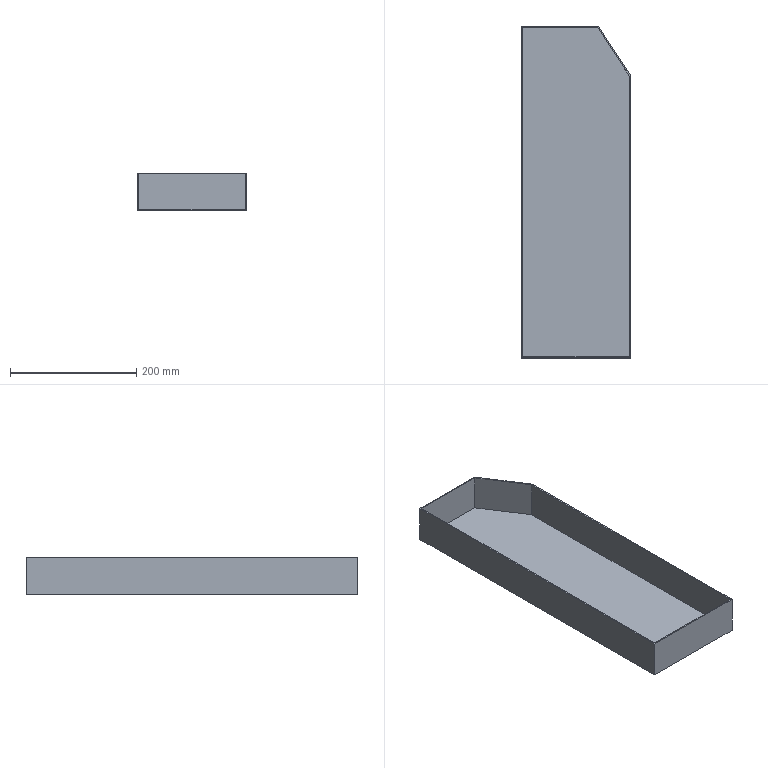Part | NX | features solid 2 | 1 solid | 13 faces | box 173 x 525 x 60 mm | volume 334513 mm3 | plane 13
STEP:
#1=CARTESIAN_POINT('',(730.,-500.,-255.));
#2=VERTEX_POINT('',#1);
#3=CARTESIAN_POINT('',(557.,-500.,-255.));
#4=VERTEX_POINT('',#3);
#5=CARTESIAN_POINT('',(-1080.,-500.,-255.));
#6=DIRECTION('',(1.,0.,0.));
#7=VECTOR('',#6,1000.);
#8=LINE('',#5,#7);
#9=EDGE_CURVE('',#2,#4,#8,.F.);
#10=ORIENTED_EDGE('',*,*,#9,.T.);
#11=CARTESIAN_POINT('',(557.,-500.,-315.));
#12=VERTEX_POINT('',#11);
#13=CARTESIAN_POINT('',(557.,-500.,-100.));
#14=DIRECTION('',(0.,0.,1.));
#15=VECTOR('',#14,1000.);
#16=LINE('',#13,#15);
#17=EDGE_CURVE('',#12,#4,#16,.T.);
#18=ORIENTED_EDGE('',*,*,#17,.F.);
#19=CARTESIAN_POINT('',(730.,-500.,-315.));
#20=VERTEX_POINT('',#19);
#21=CARTESIAN_POINT('',(-1080.,-500.,-315.));
#22=DIRECTION('',(1.,0.,0.));
#23=VECTOR('',#22,1000.);
#24=LINE('',#21,#23);
#25=EDGE_CURVE('',#20,#12,#24,.F.);
#26=ORIENTED_EDGE('',*,*,#25,.F.);
#27=CARTESIAN_POINT('',(730.,-500.,-315.));
#28=DIRECTION('',(0.,0.,1.));
#29=VECTOR('',#28,1000.);
#30=LINE('',#27,#29);
#31=EDGE_CURVE('',#20,#2,#30,.T.);
#32=ORIENTED_EDGE('',*,*,#31,.T.);
#33=EDGE_LOOP('',(#10,#18,#26,#32));
#34=FACE_BOUND('',#33,.T.);
#35=CARTESIAN_POINT('',(-1080.,-500.,-100.));
#36=DIRECTION('',(0.,1.,0.));
#37=DIRECTION('',(0.,0.,1.));
#38=AXIS2_PLACEMENT_3D('',#35,#36,#37);
#39=PLANE('',#38);
#40=ADVANCED_FACE('',(#34),#39,.F.);
#41=CARTESIAN_POINT('',(557.,25.,-255.));
#42=VERTEX_POINT('',#41);
#43=CARTESIAN_POINT('',(557.,-440.,-255.));
#44=DIRECTION('',(0.,1.,0.));
#45=VECTOR('',#44,1000.);
#46=LINE('',#43,#45);
#47=EDGE_CURVE('',#42,#4,#46,.F.);
#48=ORIENTED_EDGE('',*,*,#47,.F.);
#49=CARTESIAN_POINT('',(557.,25.,-315.));
#50=VERTEX_POINT('',#49);
#51=CARTESIAN_POINT('',(557.,25.,-315.));
#52=DIRECTION('',(0.,0.,1.));
#53=VECTOR('',#52,1000.);
#54=LINE('',#51,#53);
#55=EDGE_CURVE('',#50,#42,#54,.T.);
#56=ORIENTED_EDGE('',*,*,#55,.F.);
#57=CARTESIAN_POINT('',(557.,-440.,-315.));
#58=DIRECTION('',(0.,1.,0.));
#59=VECTOR('',#58,1000.);
#60=LINE('',#57,#59);
#61=EDGE_CURVE('',#50,#12,#60,.F.);
#62=ORIENTED_EDGE('',*,*,#61,.T.);
#63=ORIENTED_EDGE('',*,*,#17,.T.);
#64=EDGE_LOOP('',(#48,#56,#62,#63));
#65=FACE_BOUND('',#64,.T.);
#66=CARTESIAN_POINT('',(557.,-440.,-315.));
#67=DIRECTION('',(-1.,0.,0.));
#68=DIRECTION('',(0.,0.,1.));
#69=AXIS2_PLACEMENT_3D('',#66,#67,#68);
#70=PLANE('',#69);
#71=ADVANCED_FACE('',(#65),#70,.T.);
#72=CARTESIAN_POINT('',(678.942,25.,-255.));
#73=VERTEX_POINT('',#72);
#74=CARTESIAN_POINT('',(-625.,25.,-255.));
#75=DIRECTION('',(-1.,0.,0.));
#76=VECTOR('',#75,1000.);
#77=LINE('',#74,#76);
#78=EDGE_CURVE('',#42,#73,#77,.F.);
#79=ORIENTED_EDGE('',*,*,#78,.T.);
#80=CARTESIAN_POINT('',(678.942,25.,-315.));
#81=VERTEX_POINT('',#80);
#82=CARTESIAN_POINT('',(678.942,25.,-315.));
#83=DIRECTION('',(0.,0.,1.));
#84=VECTOR('',#83,1000.);
#85=LINE('',#82,#84);
#86=EDGE_CURVE('',#81,#73,#85,.T.);
#87=ORIENTED_EDGE('',*,*,#86,.F.);
#88=CARTESIAN_POINT('',(-625.,25.,-315.));
#89=DIRECTION('',(-1.,0.,0.));
#90=VECTOR('',#89,1000.);
#91=LINE('',#88,#90);
#92=EDGE_CURVE('',#50,#81,#91,.F.);
#93=ORIENTED_EDGE('',*,*,#92,.F.);
#94=ORIENTED_EDGE('',*,*,#55,.T.);
#95=EDGE_LOOP('',(#79,#87,#93,#94));
#96=FACE_BOUND('',#95,.T.);
#97=CARTESIAN_POINT('',(-625.,25.,-315.));
#98=DIRECTION('',(0.,-1.,0.));
#99=DIRECTION('',(1.,0.,0.));
#100=AXIS2_PLACEMENT_3D('',#97,#98,#99);
#101=PLANE('',#100);
#102=ADVANCED_FACE('',(#96),#101,.F.);
#103=CARTESIAN_POINT('',(730.,-53.622,-255.));
#104=VERTEX_POINT('',#103);
#105=CARTESIAN_POINT('',(628.149,103.214,-255.));
#106=DIRECTION('',(0.5446,-0.8387,0.));
#107=VECTOR('',#106,1000.);
#108=LINE('',#105,#107);
#109=EDGE_CURVE('',#104,#73,#108,.F.);
#110=ORIENTED_EDGE('',*,*,#109,.F.);
#111=CARTESIAN_POINT('',(730.,-53.622,-315.));
#112=VERTEX_POINT('',#111);
#113=CARTESIAN_POINT('',(730.,-53.622,-315.));
#114=DIRECTION('',(0.,0.,1.));
#115=VECTOR('',#114,1000.);
#116=LINE('',#113,#115);
#117=EDGE_CURVE('',#112,#104,#116,.T.);
#118=ORIENTED_EDGE('',*,*,#117,.F.);
#119=CARTESIAN_POINT('',(628.149,103.214,-315.));
#120=DIRECTION('',(0.5446,-0.8387,0.));
#121=VECTOR('',#120,1000.);
#122=LINE('',#119,#121);
#123=EDGE_CURVE('',#112,#81,#122,.F.);
#124=ORIENTED_EDGE('',*,*,#123,.T.);
#125=ORIENTED_EDGE('',*,*,#86,.T.);
#126=EDGE_LOOP('',(#110,#118,#124,#125));
#127=FACE_BOUND('',#126,.T.);
#128=CARTESIAN_POINT('',(628.149,103.214,-315.));
#129=DIRECTION('',(0.8387,0.5446,0.));
#130=DIRECTION('',(-0.5446,0.8387,0.));
#131=AXIS2_PLACEMENT_3D('',#128,#129,#130);
#132=PLANE('',#131);
#133=ADVANCED_FACE('',(#127),#132,.T.);
#134=CARTESIAN_POINT('',(730.,-550.,-255.));
#135=DIRECTION('',(0.,-1.,0.));
#136=VECTOR('',#135,1000.);
#137=LINE('',#134,#136);
#138=EDGE_CURVE('',#2,#104,#137,.F.);
#139=ORIENTED_EDGE('',*,*,#138,.F.);
#140=ORIENTED_EDGE('',*,*,#31,.F.);
#141=CARTESIAN_POINT('',(730.,-550.,-315.));
#142=DIRECTION('',(0.,-1.,0.));
#143=VECTOR('',#142,1000.);
#144=LINE('',#141,#143);
#145=EDGE_CURVE('',#20,#112,#144,.F.);
#146=ORIENTED_EDGE('',*,*,#145,.T.);
#147=ORIENTED_EDGE('',*,*,#117,.T.);
#148=EDGE_LOOP('',(#139,#140,#146,#147));
#149=FACE_BOUND('',#148,.T.);
#150=CARTESIAN_POINT('',(730.,-550.,-315.));
#151=DIRECTION('',(1.,0.,0.));
#152=DIRECTION('',(0.,0.,-1.));
#153=AXIS2_PLACEMENT_3D('',#150,#151,#152);
#154=PLANE('',#153);
#155=ADVANCED_FACE('',(#149),#154,.T.);
#156=ORIENTED_EDGE('',*,*,#25,.T.);
#157=ORIENTED_EDGE('',*,*,#61,.F.);
#158=ORIENTED_EDGE('',*,*,#92,.T.);
#159=ORIENTED_EDGE('',*,*,#123,.F.);
#160=ORIENTED_EDGE('',*,*,#145,.F.);
#161=EDGE_LOOP('',(#156,#157,#158,#159,#160));
#162=FACE_BOUND('',#161,.T.);
#163=CARTESIAN_POINT('',(1030.,-440.,-315.));
#164=DIRECTION('',(0.,0.,1.));
#165=DIRECTION('',(0.,1.,0.));
#166=AXIS2_PLACEMENT_3D('',#163,#164,#165);
#167=PLANE('',#166);
#168=ADVANCED_FACE('',(#162),#167,.F.);
#169=CARTESIAN_POINT('',(728.,-498.,-255.));
#170=VERTEX_POINT('',#169);
#171=CARTESIAN_POINT('',(728.,-54.214,-255.));
#172=VERTEX_POINT('',#171);
#173=CARTESIAN_POINT('',(728.,-550.,-255.));
#174=DIRECTION('',(0.,-1.,0.));
#175=VECTOR('',#174,1000.);
#176=LINE('',#173,#175);
#177=EDGE_CURVE('',#170,#172,#176,.F.);
#178=ORIENTED_EDGE('',*,*,#177,.F.);
#179=CARTESIAN_POINT('',(559.,-498.,-255.));
#180=VERTEX_POINT('',#179);
#181=CARTESIAN_POINT('',(-1080.,-498.,-255.));
#182=DIRECTION('',(1.,0.,0.));
#183=VECTOR('',#182,1000.);
#184=LINE('',#181,#183);
#185=EDGE_CURVE('',#170,#180,#184,.F.);
#186=ORIENTED_EDGE('',*,*,#185,.T.);
#187=CARTESIAN_POINT('',(559.,23.,-255.));
#188=VERTEX_POINT('',#187);
#189=CARTESIAN_POINT('',(559.,-440.,-255.));
#190=DIRECTION('',(0.,1.,0.));
#191=VECTOR('',#190,1000.);
#192=LINE('',#189,#191);
#193=EDGE_CURVE('',#188,#180,#192,.F.);
#194=ORIENTED_EDGE('',*,*,#193,.F.);
#195=CARTESIAN_POINT('',(677.856,23.,-255.));
#196=VERTEX_POINT('',#195);
#197=CARTESIAN_POINT('',(-625.,23.,-255.));
#198=DIRECTION('',(-1.,0.,0.));
#199=VECTOR('',#198,1000.);
#200=LINE('',#197,#199);
#201=EDGE_CURVE('',#188,#196,#200,.F.);
#202=ORIENTED_EDGE('',*,*,#201,.T.);
#203=CARTESIAN_POINT('',(626.472,102.125,-255.));
#204=DIRECTION('',(0.5446,-0.8387,0.));
#205=VECTOR('',#204,1000.);
#206=LINE('',#203,#205);
#207=EDGE_CURVE('',#172,#196,#206,.F.);
#208=ORIENTED_EDGE('',*,*,#207,.F.);
#209=EDGE_LOOP('',(#178,#186,#194,#202,#208));
#210=FACE_BOUND('',#209,.T.);
#211=ORIENTED_EDGE('',*,*,#9,.F.);
#212=ORIENTED_EDGE('',*,*,#138,.T.);
#213=ORIENTED_EDGE('',*,*,#109,.T.);
#214=ORIENTED_EDGE('',*,*,#78,.F.);
#215=ORIENTED_EDGE('',*,*,#47,.T.);
#216=EDGE_LOOP('',(#211,#212,#213,#214,#215));
#217=FACE_BOUND('',#216,.T.);
#218=CARTESIAN_POINT('',(1030.,-440.,-255.));
#219=DIRECTION('',(0.,0.,1.));
#220=DIRECTION('',(0.,1.,0.));
#221=AXIS2_PLACEMENT_3D('',#218,#219,#220);
#222=PLANE('',#221);
#223=ADVANCED_FACE('',(#210,#217),#222,.T.);
#224=ORIENTED_EDGE('',*,*,#185,.F.);
#225=CARTESIAN_POINT('',(728.,-498.,-313.));
#226=VERTEX_POINT('',#225);
#227=CARTESIAN_POINT('',(728.,-498.,-315.));
#228=DIRECTION('',(0.,0.,1.));
#229=VECTOR('',#228,1000.);
#230=LINE('',#227,#229);
#231=EDGE_CURVE('',#226,#170,#230,.T.);
#232=ORIENTED_EDGE('',*,*,#231,.F.);
#233=CARTESIAN_POINT('',(559.,-498.,-313.));
#234=VERTEX_POINT('',#233);
#235=CARTESIAN_POINT('',(-1080.,-498.,-313.));
#236=DIRECTION('',(1.,0.,0.));
#237=VECTOR('',#236,1000.);
#238=LINE('',#235,#237);
#239=EDGE_CURVE('',#226,#234,#238,.F.);
#240=ORIENTED_EDGE('',*,*,#239,.T.);
#241=CARTESIAN_POINT('',(559.,-498.,-100.));
#242=DIRECTION('',(0.,0.,1.));
#243=VECTOR('',#242,1000.);
#244=LINE('',#241,#243);
#245=EDGE_CURVE('',#234,#180,#244,.T.);
#246=ORIENTED_EDGE('',*,*,#245,.T.);
#247=EDGE_LOOP('',(#224,#232,#240,#246));
#248=FACE_BOUND('',#247,.T.);
#249=CARTESIAN_POINT('',(-1080.,-498.,-100.));
#250=DIRECTION('',(0.,1.,0.));
#251=DIRECTION('',(0.,0.,1.));
#252=AXIS2_PLACEMENT_3D('',#249,#250,#251);
#253=PLANE('',#252);
#254=ADVANCED_FACE('',(#248),#253,.T.);
#255=ORIENTED_EDGE('',*,*,#193,.T.);
#256=ORIENTED_EDGE('',*,*,#245,.F.);
#257=CARTESIAN_POINT('',(559.,23.,-313.));
#258=VERTEX_POINT('',#257);
#259=CARTESIAN_POINT('',(559.,-440.,-313.));
#260=DIRECTION('',(0.,1.,0.));
#261=VECTOR('',#260,1000.);
#262=LINE('',#259,#261);
#263=EDGE_CURVE('',#258,#234,#262,.F.);
#264=ORIENTED_EDGE('',*,*,#263,.F.);
#265=CARTESIAN_POINT('',(559.,23.,-315.));
#266=DIRECTION('',(0.,0.,1.));
#267=VECTOR('',#266,1000.);
#268=LINE('',#265,#267);
#269=EDGE_CURVE('',#258,#188,#268,.T.);
#270=ORIENTED_EDGE('',*,*,#269,.T.);
#271=EDGE_LOOP('',(#255,#256,#264,#270));
#272=FACE_BOUND('',#271,.T.);
#273=CARTESIAN_POINT('',(559.,-440.,-315.));
#274=DIRECTION('',(-1.,0.,0.));
#275=DIRECTION('',(0.,0.,1.));
#276=AXIS2_PLACEMENT_3D('',#273,#274,#275);
#277=PLANE('',#276);
#278=ADVANCED_FACE('',(#272),#277,.F.);
#279=ORIENTED_EDGE('',*,*,#201,.F.);
#280=ORIENTED_EDGE('',*,*,#269,.F.);
#281=CARTESIAN_POINT('',(677.856,23.,-313.));
#282=VERTEX_POINT('',#281);
#283=CARTESIAN_POINT('',(-625.,23.,-313.));
#284=DIRECTION('',(-1.,0.,0.));
#285=VECTOR('',#284,1000.);
#286=LINE('',#283,#285);
#287=EDGE_CURVE('',#258,#282,#286,.F.);
#288=ORIENTED_EDGE('',*,*,#287,.T.);
#289=CARTESIAN_POINT('',(677.856,23.,-315.));
#290=DIRECTION('',(0.,0.,1.));
#291=VECTOR('',#290,1000.);
#292=LINE('',#289,#291);
#293=EDGE_CURVE('',#282,#196,#292,.T.);
#294=ORIENTED_EDGE('',*,*,#293,.T.);
#295=EDGE_LOOP('',(#279,#280,#288,#294));
#296=FACE_BOUND('',#295,.T.);
#297=CARTESIAN_POINT('',(-625.,23.,-315.));
#298=DIRECTION('',(0.,-1.,0.));
#299=DIRECTION('',(1.,0.,0.));
#300=AXIS2_PLACEMENT_3D('',#297,#298,#299);
#301=PLANE('',#300);
#302=ADVANCED_FACE('',(#296),#301,.T.);
#303=ORIENTED_EDGE('',*,*,#207,.T.);
#304=ORIENTED_EDGE('',*,*,#293,.F.);
#305=CARTESIAN_POINT('',(728.,-54.214,-313.));
#306=VERTEX_POINT('',#305);
#307=CARTESIAN_POINT('',(626.472,102.125,-313.));
#308=DIRECTION('',(0.5446,-0.8387,0.));
#309=VECTOR('',#308,1000.);
#310=LINE('',#307,#309);
#311=EDGE_CURVE('',#306,#282,#310,.F.);
#312=ORIENTED_EDGE('',*,*,#311,.F.);
#313=CARTESIAN_POINT('',(728.,-54.214,-315.));
#314=DIRECTION('',(0.,0.,1.));
#315=VECTOR('',#314,1000.);
#316=LINE('',#313,#315);
#317=EDGE_CURVE('',#306,#172,#316,.T.);
#318=ORIENTED_EDGE('',*,*,#317,.T.);
#319=EDGE_LOOP('',(#303,#304,#312,#318));
#320=FACE_BOUND('',#319,.T.);
#321=CARTESIAN_POINT('',(626.472,102.125,-315.));
#322=DIRECTION('',(0.8387,0.5446,0.));
#323=DIRECTION('',(-0.5446,0.8387,0.));
#324=AXIS2_PLACEMENT_3D('',#321,#322,#323);
#325=PLANE('',#324);
#326=ADVANCED_FACE('',(#320),#325,.F.);
#327=ORIENTED_EDGE('',*,*,#177,.T.);
#328=ORIENTED_EDGE('',*,*,#317,.F.);
#329=CARTESIAN_POINT('',(728.,-550.,-313.));
#330=DIRECTION('',(0.,-1.,0.));
#331=VECTOR('',#330,1000.);
#332=LINE('',#329,#331);
#333=EDGE_CURVE('',#226,#306,#332,.F.);
#334=ORIENTED_EDGE('',*,*,#333,.F.);
#335=ORIENTED_EDGE('',*,*,#231,.T.);
#336=EDGE_LOOP('',(#327,#328,#334,#335));
#337=FACE_BOUND('',#336,.T.);
#338=CARTESIAN_POINT('',(728.,-550.,-315.));
#339=DIRECTION('',(1.,0.,0.));
#340=DIRECTION('',(0.,0.,-1.));
#341=AXIS2_PLACEMENT_3D('',#338,#339,#340);
#342=PLANE('',#341);
#343=ADVANCED_FACE('',(#337),#342,.F.);
#344=ORIENTED_EDGE('',*,*,#239,.F.);
#345=ORIENTED_EDGE('',*,*,#333,.T.);
#346=ORIENTED_EDGE('',*,*,#311,.T.);
#347=ORIENTED_EDGE('',*,*,#287,.F.);
#348=ORIENTED_EDGE('',*,*,#263,.T.);
#349=EDGE_LOOP('',(#344,#345,#346,#347,#348));
#350=FACE_BOUND('',#349,.T.);
#351=CARTESIAN_POINT('',(1030.,-440.,-313.));
#352=DIRECTION('',(0.,0.,1.));
#353=DIRECTION('',(0.,1.,0.));
#354=AXIS2_PLACEMENT_3D('',#351,#352,#353);
#355=PLANE('',#354);
#356=ADVANCED_FACE('',(#350),#355,.T.);
#357=CLOSED_SHELL('',(#40,#71,#102,#133,#155,#168,#223,#254,#278,#302,#326,#343,#356));
#358=MANIFOLD_SOLID_BREP('',#357);
#359=(LENGTH_UNIT()NAMED_UNIT(*)SI_UNIT(.MILLI.,.METRE.));
#360=UNCERTAINTY_MEASURE_WITH_UNIT(LENGTH_MEASURE(0.00001),#359,'','');
#361=(NAMED_UNIT(*)PLANE_ANGLE_UNIT()SI_UNIT($,.RADIAN.));
#362=(NAMED_UNIT(*)SI_UNIT($,.STERADIAN.)SOLID_ANGLE_UNIT());
#363=(GEOMETRIC_REPRESENTATION_CONTEXT(3)GLOBAL_UNCERTAINTY_ASSIGNED_CONTEXT((#360))GLOBAL_UNIT_ASSIGNED_CONTEXT((#359,#361,#362))REPRESENTATION_CONTEXT('',''));
#364=ADVANCED_BREP_SHAPE_REPRESENTATION('',(#358),#363);